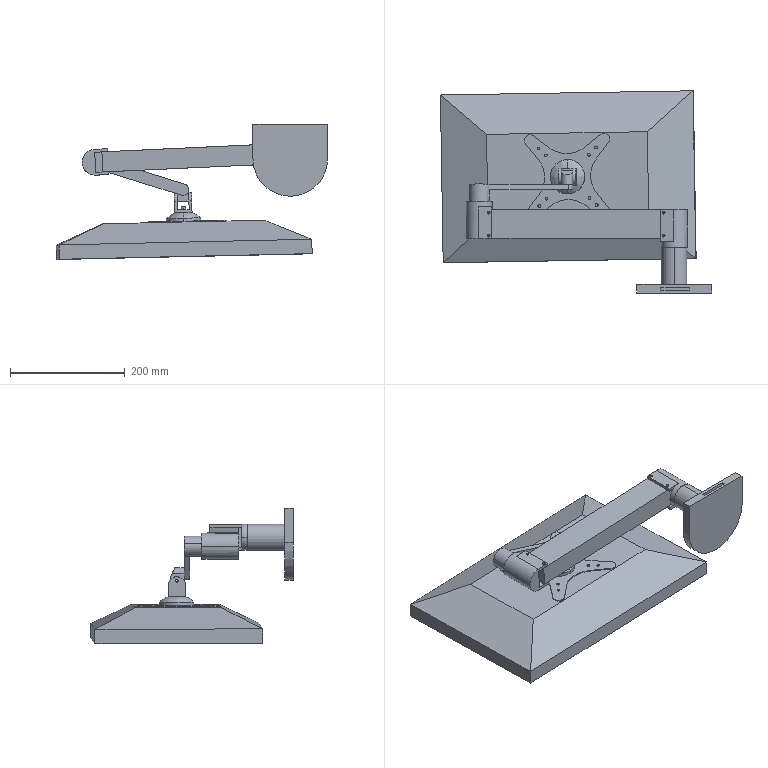Part | SolidWorks | features AEMSimFeature 1 | 9 solids | 205 faces | box 472.19 x 352.538 x 235.211 mm | volume 7182982 mm3 | cylinder 105 | plane 98 | spline 2 | commonest cylinder face diameters 5 x66 20 x10 10 x6 45 x6 100 x5 8 x4